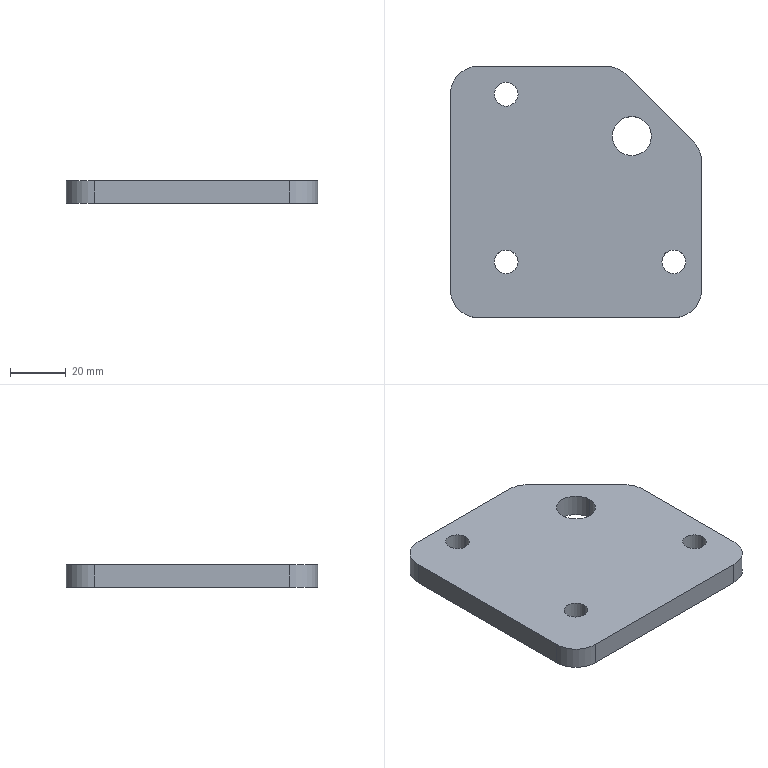Part | STEP file | 40 aluminum channel cup foot plate | 1 solid | 20 faces | box 90 x 90 x 8 mm | volume 58057 mm3 | cylinder 13 | plane 7 | commonest cylinder face diameters 8.5 x6 20 x5 14 x2